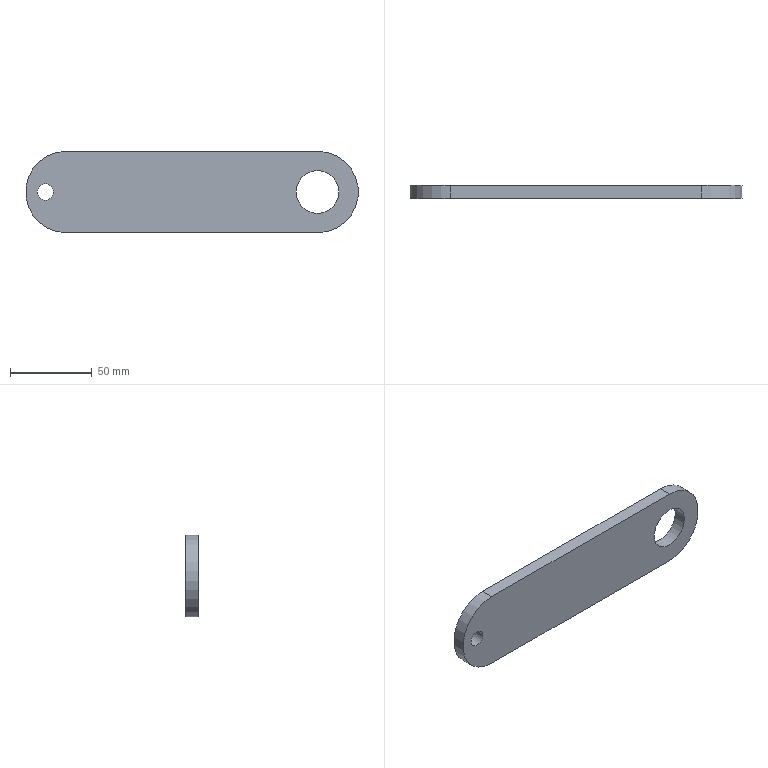Part | NX | features BREP 1 | 1 solid | 10 faces | box 203.911 x 7.95 x 49.987 mm | volume 71871 mm3 | cylinder 6 | plane 4 | commonest cylinder face diameters 10.033 x2 26.162 x2 49.987 x2
STEP:
#1=CARTESIAN_POINT('',(-76.962,0.,24.994));
#2=VERTEX_POINT('',#1);
#3=CARTESIAN_POINT('',(76.962,0.,24.994));
#4=VERTEX_POINT('',#3);
#5=CARTESIAN_POINT('',(-76.962,0.,24.994));
#6=DIRECTION('',(1.,0.,0.));
#7=VECTOR('',#6,1000.);
#8=LINE('',#5,#7);
#9=EDGE_CURVE('',#2,#4,#8,.T.);
#10=ORIENTED_EDGE('',*,*,#9,.T.);
#11=CARTESIAN_POINT('',(76.962,0.,-24.994));
#12=VERTEX_POINT('',#11);
#13=CARTESIAN_POINT('',(76.962,0.,0.));
#14=DIRECTION('',(0.,1.,0.));
#15=DIRECTION('',(0.,0.,1.));
#16=AXIS2_PLACEMENT_3D('',#13,#14,#15);
#17=CIRCLE('',#16,24.994);
#18=EDGE_CURVE('',#4,#12,#17,.T.);
#19=ORIENTED_EDGE('',*,*,#18,.T.);
#20=CARTESIAN_POINT('',(-76.962,0.,-24.994));
#21=VERTEX_POINT('',#20);
#22=CARTESIAN_POINT('',(76.962,0.,-24.994));
#23=DIRECTION('',(-1.,0.,0.));
#24=VECTOR('',#23,1000.);
#25=LINE('',#22,#24);
#26=EDGE_CURVE('',#12,#21,#25,.T.);
#27=ORIENTED_EDGE('',*,*,#26,.T.);
#28=CARTESIAN_POINT('',(-76.962,0.,0.));
#29=DIRECTION('',(0.,1.,0.));
#30=DIRECTION('',(0.,0.,-1.));
#31=AXIS2_PLACEMENT_3D('',#28,#29,#30);
#32=CIRCLE('',#31,24.994);
#33=EDGE_CURVE('',#21,#2,#32,.T.);
#34=ORIENTED_EDGE('',*,*,#33,.T.);
#35=EDGE_LOOP('',(#10,#19,#27,#34));
#36=FACE_BOUND('',#35,.T.);
#37=CARTESIAN_POINT('',(90.043,0.,0.));
#38=VERTEX_POINT('',#37);
#39=CARTESIAN_POINT('',(63.881,0.,0.));
#40=VERTEX_POINT('',#39);
#41=CARTESIAN_POINT('',(76.962,0.,0.));
#42=DIRECTION('',(0.,1.,0.));
#43=DIRECTION('',(1.,0.,0.));
#44=AXIS2_PLACEMENT_3D('',#41,#42,#43);
#45=CIRCLE('',#44,13.081);
#46=EDGE_CURVE('',#38,#40,#45,.T.);
#47=ORIENTED_EDGE('',*,*,#46,.F.);
#48=CARTESIAN_POINT('',(76.962,0.,0.));
#49=DIRECTION('',(0.,1.,0.));
#50=DIRECTION('',(-1.,0.,0.));
#51=AXIS2_PLACEMENT_3D('',#48,#49,#50);
#52=CIRCLE('',#51,13.081);
#53=EDGE_CURVE('',#40,#38,#52,.T.);
#54=ORIENTED_EDGE('',*,*,#53,.F.);
#55=EDGE_LOOP('',(#47,#54));
#56=FACE_BOUND('',#55,.T.);
#57=CARTESIAN_POINT('',(-84.9,0.,0.));
#58=VERTEX_POINT('',#57);
#59=CARTESIAN_POINT('',(-94.933,0.,0.));
#60=VERTEX_POINT('',#59);
#61=CARTESIAN_POINT('',(-89.916,0.,0.));
#62=DIRECTION('',(0.,1.,0.));
#63=DIRECTION('',(1.,0.,0.));
#64=AXIS2_PLACEMENT_3D('',#61,#62,#63);
#65=CIRCLE('',#64,5.017);
#66=EDGE_CURVE('',#58,#60,#65,.T.);
#67=ORIENTED_EDGE('',*,*,#66,.F.);
#68=CARTESIAN_POINT('',(-89.916,0.,0.));
#69=DIRECTION('',(0.,1.,0.));
#70=DIRECTION('',(-1.,0.,0.));
#71=AXIS2_PLACEMENT_3D('',#68,#69,#70);
#72=CIRCLE('',#71,5.017);
#73=EDGE_CURVE('',#60,#58,#72,.T.);
#74=ORIENTED_EDGE('',*,*,#73,.F.);
#75=EDGE_LOOP('',(#67,#74));
#76=FACE_BOUND('',#75,.T.);
#77=CARTESIAN_POINT('',(0.,0.,0.));
#78=DIRECTION('',(0.,1.,0.));
#79=DIRECTION('',(1.,0.,0.));
#80=AXIS2_PLACEMENT_3D('',#77,#78,#79);
#81=PLANE('',#80);
#82=ADVANCED_FACE('',(#36,#56,#76),#81,.T.);
#83=CARTESIAN_POINT('',(-76.962,-7.95,-24.994));
#84=VERTEX_POINT('',#83);
#85=CARTESIAN_POINT('',(-76.962,0.,-24.994));
#86=DIRECTION('',(0.,-1.,0.));
#87=VECTOR('',#86,1000.);
#88=LINE('',#85,#87);
#89=EDGE_CURVE('',#21,#84,#88,.T.);
#90=ORIENTED_EDGE('',*,*,#89,.T.);
#91=CARTESIAN_POINT('',(-76.962,-7.95,24.994));
#92=VERTEX_POINT('',#91);
#93=CARTESIAN_POINT('',(-76.962,-7.95,0.));
#94=DIRECTION('',(0.,1.,0.));
#95=DIRECTION('',(0.,0.,-1.));
#96=AXIS2_PLACEMENT_3D('',#93,#94,#95);
#97=CIRCLE('',#96,24.994);
#98=EDGE_CURVE('',#84,#92,#97,.T.);
#99=ORIENTED_EDGE('',*,*,#98,.T.);
#100=CARTESIAN_POINT('',(-76.962,0.,24.994));
#101=DIRECTION('',(0.,-1.,0.));
#102=VECTOR('',#101,1000.);
#103=LINE('',#100,#102);
#104=EDGE_CURVE('',#2,#92,#103,.T.);
#105=ORIENTED_EDGE('',*,*,#104,.F.);
#106=ORIENTED_EDGE('',*,*,#33,.F.);
#107=EDGE_LOOP('',(#90,#99,#105,#106));
#108=FACE_BOUND('',#107,.T.);
#109=CARTESIAN_POINT('',(-76.962,-3.975,0.));
#110=DIRECTION('',(0.,1.,0.));
#111=DIRECTION('',(0.,0.,-1.));
#112=AXIS2_PLACEMENT_3D('',#109,#110,#111);
#113=CYLINDRICAL_SURFACE('',#112,24.994);
#114=ADVANCED_FACE('',(#108),#113,.T.);
#115=ORIENTED_EDGE('',*,*,#104,.T.);
#116=CARTESIAN_POINT('',(76.962,-7.95,24.994));
#117=VERTEX_POINT('',#116);
#118=CARTESIAN_POINT('',(-76.962,-7.95,24.994));
#119=DIRECTION('',(1.,0.,0.));
#120=VECTOR('',#119,1000.);
#121=LINE('',#118,#120);
#122=EDGE_CURVE('',#92,#117,#121,.T.);
#123=ORIENTED_EDGE('',*,*,#122,.T.);
#124=CARTESIAN_POINT('',(76.962,0.,24.994));
#125=DIRECTION('',(0.,-1.,0.));
#126=VECTOR('',#125,1000.);
#127=LINE('',#124,#126);
#128=EDGE_CURVE('',#4,#117,#127,.T.);
#129=ORIENTED_EDGE('',*,*,#128,.F.);
#130=ORIENTED_EDGE('',*,*,#9,.F.);
#131=EDGE_LOOP('',(#115,#123,#129,#130));
#132=FACE_BOUND('',#131,.T.);
#133=CARTESIAN_POINT('',(0.,-3.975,24.994));
#134=DIRECTION('',(0.,0.,1.));
#135=DIRECTION('',(1.,0.,0.));
#136=AXIS2_PLACEMENT_3D('',#133,#134,#135);
#137=PLANE('',#136);
#138=ADVANCED_FACE('',(#132),#137,.T.);
#139=ORIENTED_EDGE('',*,*,#128,.T.);
#140=CARTESIAN_POINT('',(76.962,-7.95,-24.994));
#141=VERTEX_POINT('',#140);
#142=CARTESIAN_POINT('',(76.962,-7.95,0.));
#143=DIRECTION('',(0.,1.,0.));
#144=DIRECTION('',(0.,0.,1.));
#145=AXIS2_PLACEMENT_3D('',#142,#143,#144);
#146=CIRCLE('',#145,24.994);
#147=EDGE_CURVE('',#117,#141,#146,.T.);
#148=ORIENTED_EDGE('',*,*,#147,.T.);
#149=CARTESIAN_POINT('',(76.962,0.,-24.994));
#150=DIRECTION('',(0.,-1.,0.));
#151=VECTOR('',#150,1000.);
#152=LINE('',#149,#151);
#153=EDGE_CURVE('',#12,#141,#152,.T.);
#154=ORIENTED_EDGE('',*,*,#153,.F.);
#155=ORIENTED_EDGE('',*,*,#18,.F.);
#156=EDGE_LOOP('',(#139,#148,#154,#155));
#157=FACE_BOUND('',#156,.T.);
#158=CARTESIAN_POINT('',(76.962,-3.975,0.));
#159=DIRECTION('',(0.,1.,0.));
#160=DIRECTION('',(0.,0.,1.));
#161=AXIS2_PLACEMENT_3D('',#158,#159,#160);
#162=CYLINDRICAL_SURFACE('',#161,24.994);
#163=ADVANCED_FACE('',(#157),#162,.T.);
#164=ORIENTED_EDGE('',*,*,#153,.T.);
#165=CARTESIAN_POINT('',(76.962,-7.95,-24.994));
#166=DIRECTION('',(-1.,0.,0.));
#167=VECTOR('',#166,1000.);
#168=LINE('',#165,#167);
#169=EDGE_CURVE('',#141,#84,#168,.T.);
#170=ORIENTED_EDGE('',*,*,#169,.T.);
#171=ORIENTED_EDGE('',*,*,#89,.F.);
#172=ORIENTED_EDGE('',*,*,#26,.F.);
#173=EDGE_LOOP('',(#164,#170,#171,#172));
#174=FACE_BOUND('',#173,.T.);
#175=CARTESIAN_POINT('',(0.,-3.975,-24.994));
#176=DIRECTION('',(0.,0.,-1.));
#177=DIRECTION('',(0.,-1.,0.));
#178=AXIS2_PLACEMENT_3D('',#175,#176,#177);
#179=PLANE('',#178);
#180=ADVANCED_FACE('',(#174),#179,.T.);
#181=ORIENTED_EDGE('',*,*,#169,.F.);
#182=ORIENTED_EDGE('',*,*,#147,.F.);
#183=ORIENTED_EDGE('',*,*,#122,.F.);
#184=ORIENTED_EDGE('',*,*,#98,.F.);
#185=EDGE_LOOP('',(#181,#182,#183,#184));
#186=FACE_BOUND('',#185,.T.);
#187=CARTESIAN_POINT('',(90.043,-7.95,0.));
#188=VERTEX_POINT('',#187);
#189=CARTESIAN_POINT('',(63.881,-7.95,0.));
#190=VERTEX_POINT('',#189);
#191=CARTESIAN_POINT('',(76.962,-7.95,0.));
#192=DIRECTION('',(0.,1.,0.));
#193=DIRECTION('',(1.,0.,0.));
#194=AXIS2_PLACEMENT_3D('',#191,#192,#193);
#195=CIRCLE('',#194,13.081);
#196=EDGE_CURVE('',#188,#190,#195,.T.);
#197=ORIENTED_EDGE('',*,*,#196,.T.);
#198=CARTESIAN_POINT('',(76.962,-7.95,0.));
#199=DIRECTION('',(0.,1.,0.));
#200=DIRECTION('',(-1.,0.,0.));
#201=AXIS2_PLACEMENT_3D('',#198,#199,#200);
#202=CIRCLE('',#201,13.081);
#203=EDGE_CURVE('',#190,#188,#202,.T.);
#204=ORIENTED_EDGE('',*,*,#203,.T.);
#205=EDGE_LOOP('',(#197,#204));
#206=FACE_BOUND('',#205,.T.);
#207=CARTESIAN_POINT('',(-84.9,-7.95,0.));
#208=VERTEX_POINT('',#207);
#209=CARTESIAN_POINT('',(-94.933,-7.95,0.));
#210=VERTEX_POINT('',#209);
#211=CARTESIAN_POINT('',(-89.916,-7.95,0.));
#212=DIRECTION('',(0.,1.,0.));
#213=DIRECTION('',(1.,0.,0.));
#214=AXIS2_PLACEMENT_3D('',#211,#212,#213);
#215=CIRCLE('',#214,5.017);
#216=EDGE_CURVE('',#208,#210,#215,.T.);
#217=ORIENTED_EDGE('',*,*,#216,.T.);
#218=CARTESIAN_POINT('',(-89.916,-7.95,0.));
#219=DIRECTION('',(0.,1.,0.));
#220=DIRECTION('',(-1.,0.,0.));
#221=AXIS2_PLACEMENT_3D('',#218,#219,#220);
#222=CIRCLE('',#221,5.017);
#223=EDGE_CURVE('',#210,#208,#222,.T.);
#224=ORIENTED_EDGE('',*,*,#223,.T.);
#225=EDGE_LOOP('',(#217,#224));
#226=FACE_BOUND('',#225,.T.);
#227=CARTESIAN_POINT('',(0.,-7.95,0.));
#228=DIRECTION('',(0.,1.,0.));
#229=DIRECTION('',(1.,0.,0.));
#230=AXIS2_PLACEMENT_3D('',#227,#228,#229);
#231=PLANE('',#230);
#232=ADVANCED_FACE('',(#186,#206,#226),#231,.F.);
#233=CARTESIAN_POINT('',(90.043,0.,0.));
#234=DIRECTION('',(0.,-1.,0.));
#235=VECTOR('',#234,1000.);
#236=LINE('',#233,#235);
#237=EDGE_CURVE('',#188,#38,#236,.F.);
#238=ORIENTED_EDGE('',*,*,#237,.F.);
#239=ORIENTED_EDGE('',*,*,#203,.F.);
#240=CARTESIAN_POINT('',(63.881,0.,0.));
#241=DIRECTION('',(0.,-1.,0.));
#242=VECTOR('',#241,1000.);
#243=LINE('',#240,#242);
#244=EDGE_CURVE('',#190,#40,#243,.F.);
#245=ORIENTED_EDGE('',*,*,#244,.T.);
#246=ORIENTED_EDGE('',*,*,#53,.T.);
#247=EDGE_LOOP('',(#238,#239,#245,#246));
#248=FACE_BOUND('',#247,.T.);
#249=CARTESIAN_POINT('',(76.962,-3.975,0.));
#250=DIRECTION('',(0.,1.,0.));
#251=DIRECTION('',(-1.,0.,0.));
#252=AXIS2_PLACEMENT_3D('',#249,#250,#251);
#253=CYLINDRICAL_SURFACE('',#252,13.081);
#254=ADVANCED_FACE('',(#248),#253,.F.);
#255=ORIENTED_EDGE('',*,*,#244,.F.);
#256=ORIENTED_EDGE('',*,*,#196,.F.);
#257=ORIENTED_EDGE('',*,*,#237,.T.);
#258=ORIENTED_EDGE('',*,*,#46,.T.);
#259=EDGE_LOOP('',(#255,#256,#257,#258));
#260=FACE_BOUND('',#259,.T.);
#261=CARTESIAN_POINT('',(76.962,-3.975,0.));
#262=DIRECTION('',(0.,1.,0.));
#263=DIRECTION('',(1.,0.,0.));
#264=AXIS2_PLACEMENT_3D('',#261,#262,#263);
#265=CYLINDRICAL_SURFACE('',#264,13.081);
#266=ADVANCED_FACE('',(#260),#265,.F.);
#267=CARTESIAN_POINT('',(-84.9,0.,0.));
#268=DIRECTION('',(0.,-1.,0.));
#269=VECTOR('',#268,1000.);
#270=LINE('',#267,#269);
#271=EDGE_CURVE('',#208,#58,#270,.F.);
#272=ORIENTED_EDGE('',*,*,#271,.F.);
#273=ORIENTED_EDGE('',*,*,#223,.F.);
#274=CARTESIAN_POINT('',(-94.933,0.,0.));
#275=DIRECTION('',(0.,-1.,0.));
#276=VECTOR('',#275,1000.);
#277=LINE('',#274,#276);
#278=EDGE_CURVE('',#210,#60,#277,.F.);
#279=ORIENTED_EDGE('',*,*,#278,.T.);
#280=ORIENTED_EDGE('',*,*,#73,.T.);
#281=EDGE_LOOP('',(#272,#273,#279,#280));
#282=FACE_BOUND('',#281,.T.);
#283=CARTESIAN_POINT('',(-89.916,-3.975,0.));
#284=DIRECTION('',(0.,1.,0.));
#285=DIRECTION('',(-1.,0.,0.));
#286=AXIS2_PLACEMENT_3D('',#283,#284,#285);
#287=CYLINDRICAL_SURFACE('',#286,5.017);
#288=ADVANCED_FACE('',(#282),#287,.F.);
#289=ORIENTED_EDGE('',*,*,#278,.F.);
#290=ORIENTED_EDGE('',*,*,#216,.F.);
#291=ORIENTED_EDGE('',*,*,#271,.T.);
#292=ORIENTED_EDGE('',*,*,#66,.T.);
#293=EDGE_LOOP('',(#289,#290,#291,#292));
#294=FACE_BOUND('',#293,.T.);
#295=CARTESIAN_POINT('',(-89.916,-3.975,0.));
#296=DIRECTION('',(0.,1.,0.));
#297=DIRECTION('',(1.,0.,0.));
#298=AXIS2_PLACEMENT_3D('',#295,#296,#297);
#299=CYLINDRICAL_SURFACE('',#298,5.017);
#300=ADVANCED_FACE('',(#294),#299,.F.);
#301=CLOSED_SHELL('',(#82,#114,#138,#163,#180,#232,#254,#266,#288,#300));
#302=MANIFOLD_SOLID_BREP('',#301);
#303=(LENGTH_UNIT()NAMED_UNIT(*)SI_UNIT(.MILLI.,.METRE.));
#304=UNCERTAINTY_MEASURE_WITH_UNIT(LENGTH_MEASURE(0.00001),#303,'','');
#305=(NAMED_UNIT(*)PLANE_ANGLE_UNIT()SI_UNIT($,.RADIAN.));
#306=(NAMED_UNIT(*)SI_UNIT($,.STERADIAN.)SOLID_ANGLE_UNIT());
#307=(GEOMETRIC_REPRESENTATION_CONTEXT(3)GLOBAL_UNCERTAINTY_ASSIGNED_CONTEXT((#304))GLOBAL_UNIT_ASSIGNED_CONTEXT((#303,#305,#306))REPRESENTATION_CONTEXT('',''));
#308=ADVANCED_BREP_SHAPE_REPRESENTATION('',(#302),#307);